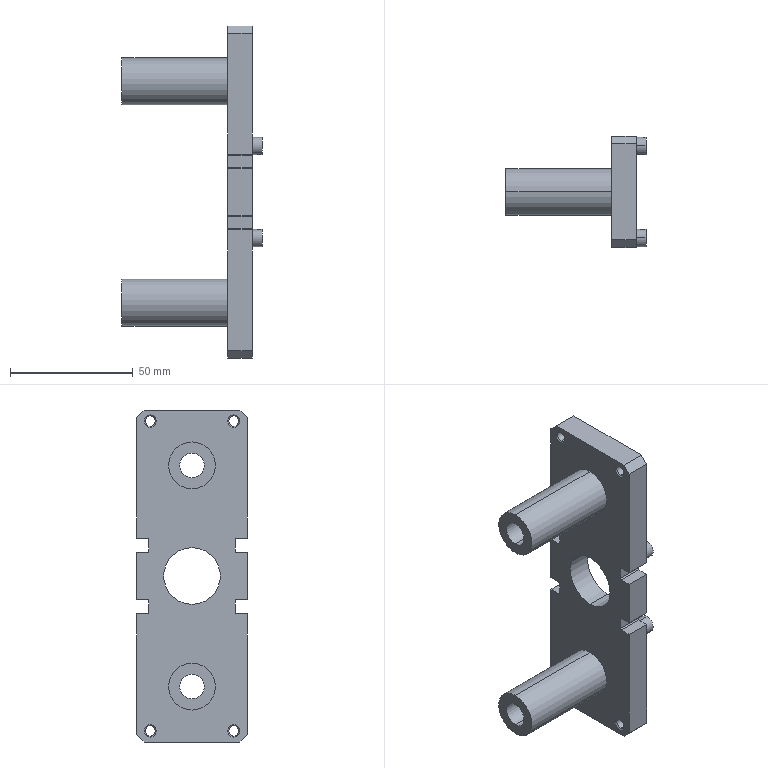Part | STEP file | Guide wheel mechanism revised.sldasm-Part-472 | 1 solid | 86 faces | box 57 x 45 x 135 mm | volume 71386 mm3 | plane 36 | cylinder 34 | cone 16 | commonest cylinder face diameters 1 x8 4.134 x8 7 x8 10 x4 19 x4 23 x2